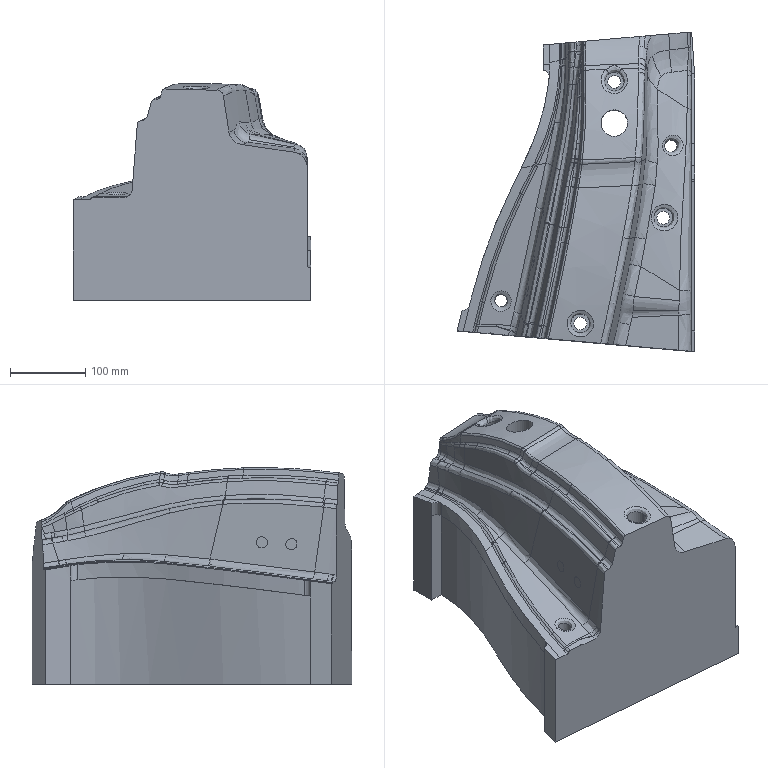Part | NX | features solid 2 | 1 solid | 239 faces | box 315.294 x 423.565 x 287.118 mm | volume 20643324 mm3 | spline 213 | plane 13 | cylinder 13 | commonest cylinder face diameters 17 x5 25 x3 16 x2 20 x2 35 x1